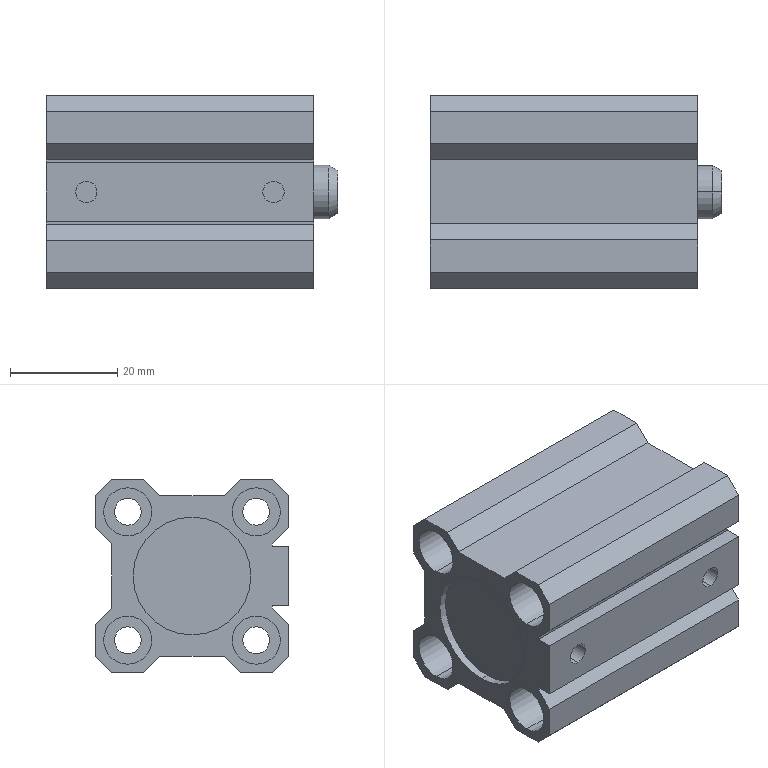Part | STEP file | Air Cylinder CQ2B20-30DC | 1 solid | 85 faces | box 54.5 x 36 x 36 mm | volume 48635 mm3 | plane 45 | cylinder 38 | cone 2 | commonest cylinder face diameters 9 x16 5 x10 4 x4 22 x4 10 x2 13 x2